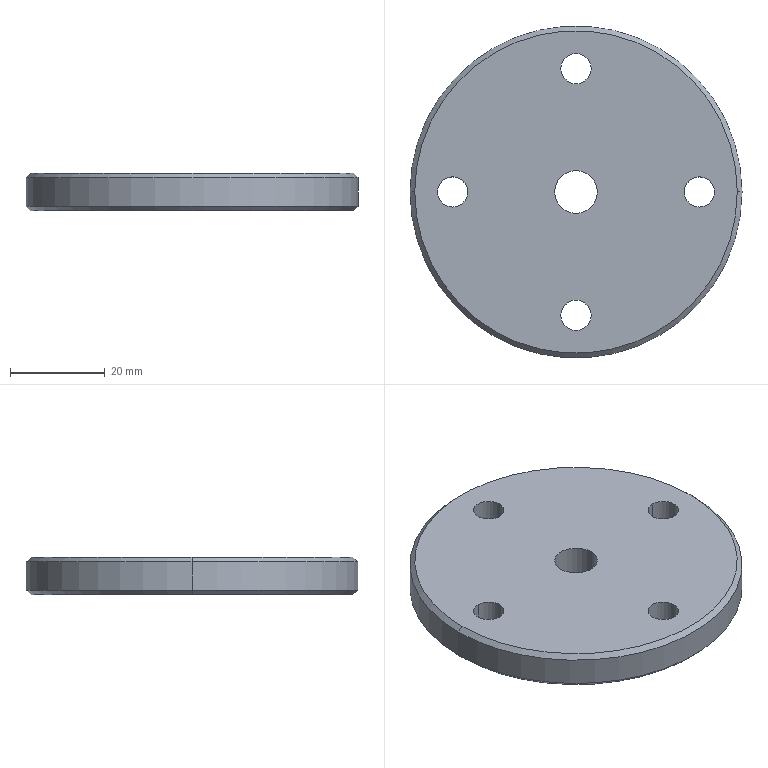Part | NX | features BREP 1 | 1 solid | 18 faces | box 70 x 70 x 8 mm | volume 29031 mm3 | cylinder 12 | cone 4 | plane 2 | commonest cylinder face diameters 6.4 x8 9 x2 70 x2
STEP:
#1=CARTESIAN_POINT('',(3.2,-26.,8.));
#2=VERTEX_POINT('',#1);
#3=CARTESIAN_POINT('',(-3.2,-26.,8.));
#4=VERTEX_POINT('',#3);
#5=CARTESIAN_POINT('',(0.,-26.,8.));
#6=DIRECTION('',(0.,0.,-1.));
#7=DIRECTION('',(1.,0.,0.));
#8=AXIS2_PLACEMENT_3D('',#5,#6,#7);
#9=CIRCLE('',#8,3.2);
#10=EDGE_CURVE('',#2,#4,#9,.T.);
#11=ORIENTED_EDGE('',*,*,#10,.F.);
#12=CARTESIAN_POINT('',(3.2,-26.,0.));
#13=VERTEX_POINT('',#12);
#14=CARTESIAN_POINT('',(3.2,-26.,0.));
#15=DIRECTION('',(0.,0.,1.));
#16=VECTOR('',#15,1000.);
#17=LINE('',#14,#16);
#18=EDGE_CURVE('',#2,#13,#17,.F.);
#19=ORIENTED_EDGE('',*,*,#18,.T.);
#20=CARTESIAN_POINT('',(-3.2,-26.,0.));
#21=VERTEX_POINT('',#20);
#22=CARTESIAN_POINT('',(0.,-26.,0.));
#23=DIRECTION('',(0.,0.,1.));
#24=DIRECTION('',(-1.,0.,0.));
#25=AXIS2_PLACEMENT_3D('',#22,#23,#24);
#26=CIRCLE('',#25,3.2);
#27=EDGE_CURVE('',#21,#13,#26,.T.);
#28=ORIENTED_EDGE('',*,*,#27,.F.);
#29=CARTESIAN_POINT('',(-3.2,-26.,0.));
#30=DIRECTION('',(0.,0.,1.));
#31=VECTOR('',#30,1000.);
#32=LINE('',#29,#31);
#33=EDGE_CURVE('',#4,#21,#32,.F.);
#34=ORIENTED_EDGE('',*,*,#33,.F.);
#35=EDGE_LOOP('',(#11,#19,#28,#34));
#36=FACE_BOUND('',#35,.T.);
#37=CARTESIAN_POINT('',(0.,-26.,0.));
#38=DIRECTION('',(0.,0.,1.));
#39=DIRECTION('',(1.,0.,0.));
#40=AXIS2_PLACEMENT_3D('',#37,#38,#39);
#41=CYLINDRICAL_SURFACE('',#40,3.2);
#42=ADVANCED_FACE('',(#36),#41,.F.);
#43=CARTESIAN_POINT('',(0.,-26.,8.));
#44=DIRECTION('',(0.,0.,-1.));
#45=DIRECTION('',(-1.,0.,0.));
#46=AXIS2_PLACEMENT_3D('',#43,#44,#45);
#47=CIRCLE('',#46,3.2);
#48=EDGE_CURVE('',#4,#2,#47,.T.);
#49=ORIENTED_EDGE('',*,*,#48,.F.);
#50=ORIENTED_EDGE('',*,*,#33,.T.);
#51=CARTESIAN_POINT('',(0.,-26.,0.));
#52=DIRECTION('',(0.,0.,1.));
#53=DIRECTION('',(1.,0.,0.));
#54=AXIS2_PLACEMENT_3D('',#51,#52,#53);
#55=CIRCLE('',#54,3.2);
#56=EDGE_CURVE('',#13,#21,#55,.T.);
#57=ORIENTED_EDGE('',*,*,#56,.F.);
#58=ORIENTED_EDGE('',*,*,#18,.F.);
#59=EDGE_LOOP('',(#49,#50,#57,#58));
#60=FACE_BOUND('',#59,.T.);
#61=CARTESIAN_POINT('',(0.,-26.,0.));
#62=DIRECTION('',(0.,0.,1.));
#63=DIRECTION('',(1.,0.,0.));
#64=AXIS2_PLACEMENT_3D('',#61,#62,#63);
#65=CYLINDRICAL_SURFACE('',#64,3.2);
#66=ADVANCED_FACE('',(#60),#65,.F.);
#67=CARTESIAN_POINT('',(34.,-0.000000001,0.));
#68=VERTEX_POINT('',#67);
#69=CARTESIAN_POINT('',(-34.,0.,0.));
#70=VERTEX_POINT('',#69);
#71=CARTESIAN_POINT('',(0.,0.,0.));
#72=DIRECTION('',(0.,0.,-1.));
#73=DIRECTION('',(0.5,-0.866,0.));
#74=AXIS2_PLACEMENT_3D('',#71,#72,#73);
#75=CIRCLE('',#74,34.);
#76=EDGE_CURVE('',#68,#70,#75,.T.);
#77=ORIENTED_EDGE('',*,*,#76,.T.);
#78=CARTESIAN_POINT('',(0.,0.,0.));
#79=DIRECTION('',(0.,0.,-1.));
#80=DIRECTION('',(-1.,0.,0.));
#81=AXIS2_PLACEMENT_3D('',#78,#79,#80);
#82=CIRCLE('',#81,34.);
#83=EDGE_CURVE('',#70,#68,#82,.T.);
#84=ORIENTED_EDGE('',*,*,#83,.T.);
#85=EDGE_LOOP('',(#77,#84));
#86=FACE_BOUND('',#85,.T.);
#87=ORIENTED_EDGE('',*,*,#56,.T.);
#88=ORIENTED_EDGE('',*,*,#27,.T.);
#89=EDGE_LOOP('',(#87,#88));
#90=FACE_BOUND('',#89,.T.);
#91=CARTESIAN_POINT('',(4.5,0.,0.));
#92=VERTEX_POINT('',#91);
#93=CARTESIAN_POINT('',(-4.5,0.,0.));
#94=VERTEX_POINT('',#93);
#95=CARTESIAN_POINT('',(0.,0.,0.));
#96=DIRECTION('',(0.,0.,1.));
#97=DIRECTION('',(1.,0.,0.));
#98=AXIS2_PLACEMENT_3D('',#95,#96,#97);
#99=CIRCLE('',#98,4.5);
#100=EDGE_CURVE('',#92,#94,#99,.T.);
#101=ORIENTED_EDGE('',*,*,#100,.T.);
#102=CARTESIAN_POINT('',(0.,0.,0.));
#103=DIRECTION('',(0.,0.,1.));
#104=DIRECTION('',(-1.,0.,0.));
#105=AXIS2_PLACEMENT_3D('',#102,#103,#104);
#106=CIRCLE('',#105,4.5);
#107=EDGE_CURVE('',#94,#92,#106,.T.);
#108=ORIENTED_EDGE('',*,*,#107,.T.);
#109=EDGE_LOOP('',(#101,#108));
#110=FACE_BOUND('',#109,.T.);
#111=CARTESIAN_POINT('',(26.,3.2,0.));
#112=VERTEX_POINT('',#111);
#113=CARTESIAN_POINT('',(26.,-3.2,0.));
#114=VERTEX_POINT('',#113);
#115=CARTESIAN_POINT('',(26.,0.,0.));
#116=DIRECTION('',(0.,0.,1.));
#117=DIRECTION('',(-1.,0.,0.));
#118=AXIS2_PLACEMENT_3D('',#115,#116,#117);
#119=CIRCLE('',#118,3.2);
#120=EDGE_CURVE('',#112,#114,#119,.T.);
#121=ORIENTED_EDGE('',*,*,#120,.T.);
#122=CARTESIAN_POINT('',(26.,0.,0.));
#123=DIRECTION('',(0.,0.,1.));
#124=DIRECTION('',(0.,-1.,0.));
#125=AXIS2_PLACEMENT_3D('',#122,#123,#124);
#126=CIRCLE('',#125,3.2);
#127=EDGE_CURVE('',#114,#112,#126,.T.);
#128=ORIENTED_EDGE('',*,*,#127,.T.);
#129=EDGE_LOOP('',(#121,#128));
#130=FACE_BOUND('',#129,.T.);
#131=CARTESIAN_POINT('',(3.2,26.,0.));
#132=VERTEX_POINT('',#131);
#133=CARTESIAN_POINT('',(-3.2,26.,0.));
#134=VERTEX_POINT('',#133);
#135=CARTESIAN_POINT('',(0.,26.,0.));
#136=DIRECTION('',(0.,0.,1.));
#137=DIRECTION('',(1.,0.,0.));
#138=AXIS2_PLACEMENT_3D('',#135,#136,#137);
#139=CIRCLE('',#138,3.2);
#140=EDGE_CURVE('',#132,#134,#139,.T.);
#141=ORIENTED_EDGE('',*,*,#140,.T.);
#142=CARTESIAN_POINT('',(0.,26.,0.));
#143=DIRECTION('',(0.,0.,1.));
#144=DIRECTION('',(-1.,0.,0.));
#145=AXIS2_PLACEMENT_3D('',#142,#143,#144);
#146=CIRCLE('',#145,3.2);
#147=EDGE_CURVE('',#134,#132,#146,.T.);
#148=ORIENTED_EDGE('',*,*,#147,.T.);
#149=EDGE_LOOP('',(#141,#148));
#150=FACE_BOUND('',#149,.T.);
#151=CARTESIAN_POINT('',(-26.,3.2,0.));
#152=VERTEX_POINT('',#151);
#153=CARTESIAN_POINT('',(-26.,-3.2,0.));
#154=VERTEX_POINT('',#153);
#155=CARTESIAN_POINT('',(-26.,0.,0.));
#156=DIRECTION('',(0.,0.,1.));
#157=DIRECTION('',(0.,1.,0.));
#158=AXIS2_PLACEMENT_3D('',#155,#156,#157);
#159=CIRCLE('',#158,3.2);
#160=EDGE_CURVE('',#152,#154,#159,.T.);
#161=ORIENTED_EDGE('',*,*,#160,.T.);
#162=CARTESIAN_POINT('',(-26.,0.,0.));
#163=DIRECTION('',(0.,0.,1.));
#164=DIRECTION('',(0.,-1.,0.));
#165=AXIS2_PLACEMENT_3D('',#162,#163,#164);
#166=CIRCLE('',#165,3.2);
#167=EDGE_CURVE('',#154,#152,#166,.T.);
#168=ORIENTED_EDGE('',*,*,#167,.T.);
#169=EDGE_LOOP('',(#161,#168));
#170=FACE_BOUND('',#169,.T.);
#171=CARTESIAN_POINT('',(0.,0.,0.));
#172=DIRECTION('',(0.,0.,1.));
#173=DIRECTION('',(1.,0.,0.));
#174=AXIS2_PLACEMENT_3D('',#171,#172,#173);
#175=PLANE('',#174);
#176=ADVANCED_FACE('',(#86,#90,#110,#130,#150,#170),#175,.F.);
#177=CARTESIAN_POINT('',(35.,0.,1.));
#178=VERTEX_POINT('',#177);
#179=CARTESIAN_POINT('',(35.,0.,1.));
#180=DIRECTION('',(-0.7071,0.,-0.7071));
#181=VECTOR('',#180,1000.);
#182=LINE('',#179,#181);
#183=EDGE_CURVE('',#68,#178,#182,.F.);
#184=ORIENTED_EDGE('',*,*,#183,.T.);
#185=CARTESIAN_POINT('',(-35.,0.,1.));
#186=VERTEX_POINT('',#185);
#187=CARTESIAN_POINT('',(0.,0.,1.));
#188=DIRECTION('',(0.,0.,-1.));
#189=DIRECTION('',(1.,0.,0.));
#190=AXIS2_PLACEMENT_3D('',#187,#188,#189);
#191=CIRCLE('',#190,35.);
#192=EDGE_CURVE('',#178,#186,#191,.T.);
#193=ORIENTED_EDGE('',*,*,#192,.T.);
#194=CARTESIAN_POINT('',(-35.,0.,1.));
#195=DIRECTION('',(0.7071,0.,-0.7071));
#196=VECTOR('',#195,1000.);
#197=LINE('',#194,#196);
#198=EDGE_CURVE('',#70,#186,#197,.F.);
#199=ORIENTED_EDGE('',*,*,#198,.F.);
#200=ORIENTED_EDGE('',*,*,#76,.F.);
#201=EDGE_LOOP('',(#184,#193,#199,#200));
#202=FACE_BOUND('',#201,.T.);
#203=CARTESIAN_POINT('',(0.,0.,0.5));
#204=DIRECTION('',(0.,0.,1.));
#205=DIRECTION('',(1.,0.,0.));
#206=AXIS2_PLACEMENT_3D('',#203,#204,#205);
#207=CONICAL_SURFACE('',#206,34.5,0.7854);
#208=ADVANCED_FACE('',(#202),#207,.T.);
#209=ORIENTED_EDGE('',*,*,#83,.F.);
#210=ORIENTED_EDGE('',*,*,#198,.T.);
#211=CARTESIAN_POINT('',(0.,0.,1.));
#212=DIRECTION('',(0.,0.,-1.));
#213=DIRECTION('',(-1.,0.,0.));
#214=AXIS2_PLACEMENT_3D('',#211,#212,#213);
#215=CIRCLE('',#214,35.);
#216=EDGE_CURVE('',#186,#178,#215,.T.);
#217=ORIENTED_EDGE('',*,*,#216,.T.);
#218=ORIENTED_EDGE('',*,*,#183,.F.);
#219=EDGE_LOOP('',(#209,#210,#217,#218));
#220=FACE_BOUND('',#219,.T.);
#221=CARTESIAN_POINT('',(0.,0.,0.5));
#222=DIRECTION('',(0.,0.,1.));
#223=DIRECTION('',(1.,0.,0.));
#224=AXIS2_PLACEMENT_3D('',#221,#222,#223);
#225=CONICAL_SURFACE('',#224,34.5,0.7854);
#226=ADVANCED_FACE('',(#220),#225,.T.);
#227=ORIENTED_EDGE('',*,*,#216,.F.);
#228=CARTESIAN_POINT('',(-35.,0.,7.));
#229=VERTEX_POINT('',#228);
#230=CARTESIAN_POINT('',(-35.,0.,7.));
#231=DIRECTION('',(0.,0.,-1.));
#232=VECTOR('',#231,1000.);
#233=LINE('',#230,#232);
#234=EDGE_CURVE('',#186,#229,#233,.F.);
#235=ORIENTED_EDGE('',*,*,#234,.T.);
#236=CARTESIAN_POINT('',(35.,0.,7.));
#237=VERTEX_POINT('',#236);
#238=CARTESIAN_POINT('',(0.,0.,7.));
#239=DIRECTION('',(0.,0.,1.));
#240=DIRECTION('',(1.,0.,0.));
#241=AXIS2_PLACEMENT_3D('',#238,#239,#240);
#242=CIRCLE('',#241,35.);
#243=EDGE_CURVE('',#237,#229,#242,.T.);
#244=ORIENTED_EDGE('',*,*,#243,.F.);
#245=CARTESIAN_POINT('',(35.,0.,7.));
#246=DIRECTION('',(0.,0.,-1.));
#247=VECTOR('',#246,1000.);
#248=LINE('',#245,#247);
#249=EDGE_CURVE('',#178,#237,#248,.F.);
#250=ORIENTED_EDGE('',*,*,#249,.F.);
#251=EDGE_LOOP('',(#227,#235,#244,#250));
#252=FACE_BOUND('',#251,.T.);
#253=CARTESIAN_POINT('',(0.,0.,4.));
#254=DIRECTION('',(0.,0.,1.));
#255=DIRECTION('',(1.,0.,0.));
#256=AXIS2_PLACEMENT_3D('',#253,#254,#255);
#257=CYLINDRICAL_SURFACE('',#256,35.);
#258=ADVANCED_FACE('',(#252),#257,.T.);
#259=ORIENTED_EDGE('',*,*,#234,.F.);
#260=ORIENTED_EDGE('',*,*,#192,.F.);
#261=ORIENTED_EDGE('',*,*,#249,.T.);
#262=CARTESIAN_POINT('',(0.,0.,7.));
#263=DIRECTION('',(0.,0.,1.));
#264=DIRECTION('',(0.5,-0.866,0.));
#265=AXIS2_PLACEMENT_3D('',#262,#263,#264);
#266=CIRCLE('',#265,35.);
#267=EDGE_CURVE('',#229,#237,#266,.T.);
#268=ORIENTED_EDGE('',*,*,#267,.F.);
#269=EDGE_LOOP('',(#259,#260,#261,#268));
#270=FACE_BOUND('',#269,.T.);
#271=CARTESIAN_POINT('',(0.,0.,4.));
#272=DIRECTION('',(0.,0.,1.));
#273=DIRECTION('',(1.,0.,0.));
#274=AXIS2_PLACEMENT_3D('',#271,#272,#273);
#275=CYLINDRICAL_SURFACE('',#274,35.);
#276=ADVANCED_FACE('',(#270),#275,.T.);
#277=CARTESIAN_POINT('',(-34.,0.,8.));
#278=VERTEX_POINT('',#277);
#279=CARTESIAN_POINT('',(-34.,0.,8.));
#280=DIRECTION('',(-0.7071,0.,-0.7071));
#281=VECTOR('',#280,1000.);
#282=LINE('',#279,#281);
#283=EDGE_CURVE('',#278,#229,#282,.T.);
#284=ORIENTED_EDGE('',*,*,#283,.T.);
#285=ORIENTED_EDGE('',*,*,#267,.T.);
#286=CARTESIAN_POINT('',(34.,0.,8.));
#287=VERTEX_POINT('',#286);
#288=CARTESIAN_POINT('',(35.,0.,7.));
#289=DIRECTION('',(-0.7071,0.,0.7071));
#290=VECTOR('',#289,1000.);
#291=LINE('',#288,#290);
#292=EDGE_CURVE('',#237,#287,#291,.T.);
#293=ORIENTED_EDGE('',*,*,#292,.T.);
#294=CARTESIAN_POINT('',(0.,0.,8.));
#295=DIRECTION('',(0.,0.,1.));
#296=DIRECTION('',(0.5,-0.866,0.));
#297=AXIS2_PLACEMENT_3D('',#294,#295,#296);
#298=CIRCLE('',#297,34.);
#299=EDGE_CURVE('',#278,#287,#298,.T.);
#300=ORIENTED_EDGE('',*,*,#299,.F.);
#301=EDGE_LOOP('',(#284,#285,#293,#300));
#302=FACE_BOUND('',#301,.T.);
#303=CARTESIAN_POINT('',(0.,0.,7.5));
#304=DIRECTION('',(0.,0.,-1.));
#305=DIRECTION('',(1.,0.,0.));
#306=AXIS2_PLACEMENT_3D('',#303,#304,#305);
#307=CONICAL_SURFACE('',#306,34.5,0.7854);
#308=ADVANCED_FACE('',(#302),#307,.T.);
#309=CARTESIAN_POINT('',(0.,0.,8.));
#310=DIRECTION('',(0.,0.,1.));
#311=DIRECTION('',(1.,0.,0.));
#312=AXIS2_PLACEMENT_3D('',#309,#310,#311);
#313=CIRCLE('',#312,34.);
#314=EDGE_CURVE('',#287,#278,#313,.T.);
#315=ORIENTED_EDGE('',*,*,#314,.T.);
#316=ORIENTED_EDGE('',*,*,#299,.T.);
#317=EDGE_LOOP('',(#315,#316));
#318=FACE_BOUND('',#317,.T.);
#319=ORIENTED_EDGE('',*,*,#10,.T.);
#320=ORIENTED_EDGE('',*,*,#48,.T.);
#321=EDGE_LOOP('',(#319,#320));
#322=FACE_BOUND('',#321,.T.);
#323=CARTESIAN_POINT('',(4.5,0.,8.));
#324=VERTEX_POINT('',#323);
#325=CARTESIAN_POINT('',(-4.5,0.,8.));
#326=VERTEX_POINT('',#325);
#327=CARTESIAN_POINT('',(0.,0.,8.));
#328=DIRECTION('',(0.,0.,-1.));
#329=DIRECTION('',(1.,0.,0.));
#330=AXIS2_PLACEMENT_3D('',#327,#328,#329);
#331=CIRCLE('',#330,4.5);
#332=EDGE_CURVE('',#324,#326,#331,.T.);
#333=ORIENTED_EDGE('',*,*,#332,.T.);
#334=CARTESIAN_POINT('',(0.,0.,8.));
#335=DIRECTION('',(0.,0.,-1.));
#336=DIRECTION('',(-1.,0.,0.));
#337=AXIS2_PLACEMENT_3D('',#334,#335,#336);
#338=CIRCLE('',#337,4.5);
#339=EDGE_CURVE('',#326,#324,#338,.T.);
#340=ORIENTED_EDGE('',*,*,#339,.T.);
#341=EDGE_LOOP('',(#333,#340));
#342=FACE_BOUND('',#341,.T.);
#343=CARTESIAN_POINT('',(26.,-3.2,8.));
#344=VERTEX_POINT('',#343);
#345=CARTESIAN_POINT('',(26.,3.2,8.));
#346=VERTEX_POINT('',#345);
#347=CARTESIAN_POINT('',(26.,0.,8.));
#348=DIRECTION('',(0.,0.,-1.));
#349=DIRECTION('',(0.,-1.,0.));
#350=AXIS2_PLACEMENT_3D('',#347,#348,#349);
#351=CIRCLE('',#350,3.2);
#352=EDGE_CURVE('',#344,#346,#351,.T.);
#353=ORIENTED_EDGE('',*,*,#352,.T.);
#354=CARTESIAN_POINT('',(26.,0.,8.));
#355=DIRECTION('',(0.,0.,-1.));
#356=DIRECTION('',(0.,1.,0.));
#357=AXIS2_PLACEMENT_3D('',#354,#355,#356);
#358=CIRCLE('',#357,3.2);
#359=EDGE_CURVE('',#346,#344,#358,.T.);
#360=ORIENTED_EDGE('',*,*,#359,.T.);
#361=EDGE_LOOP('',(#353,#360));
#362=FACE_BOUND('',#361,.T.);
#363=CARTESIAN_POINT('',(3.2,26.,8.));
#364=VERTEX_POINT('',#363);
#365=CARTESIAN_POINT('',(-3.2,26.,8.));
#366=VERTEX_POINT('',#365);
#367=CARTESIAN_POINT('',(0.,26.,8.));
#368=DIRECTION('',(0.,0.,-1.));
#369=DIRECTION('',(1.,0.,0.));
#370=AXIS2_PLACEMENT_3D('',#367,#368,#369);
#371=CIRCLE('',#370,3.2);
#372=EDGE_CURVE('',#364,#366,#371,.T.);
#373=ORIENTED_EDGE('',*,*,#372,.T.);
#374=CARTESIAN_POINT('',(0.,26.,8.));
#375=DIRECTION('',(0.,0.,-1.));
#376=DIRECTION('',(-1.,0.,0.));
#377=AXIS2_PLACEMENT_3D('',#374,#375,#376);
#378=CIRCLE('',#377,3.2);
#379=EDGE_CURVE('',#366,#364,#378,.T.);
#380=ORIENTED_EDGE('',*,*,#379,.T.);
#381=EDGE_LOOP('',(#373,#380));
#382=FACE_BOUND('',#381,.T.);
#383=CARTESIAN_POINT('',(-26.,3.2,8.));
#384=VERTEX_POINT('',#383);
#385=CARTESIAN_POINT('',(-26.,-3.2,8.));
#386=VERTEX_POINT('',#385);
#387=CARTESIAN_POINT('',(-26.,0.,8.));
#388=DIRECTION('',(0.,0.,-1.));
#389=DIRECTION('',(0.,1.,0.));
#390=AXIS2_PLACEMENT_3D('',#387,#388,#389);
#391=CIRCLE('',#390,3.2);
#392=EDGE_CURVE('',#384,#386,#391,.T.);
#393=ORIENTED_EDGE('',*,*,#392,.T.);
#394=CARTESIAN_POINT('',(-26.,0.,8.));
#395=DIRECTION('',(0.,0.,-1.));
#396=DIRECTION('',(0.,-1.,0.));
#397=AXIS2_PLACEMENT_3D('',#394,#395,#396);
#398=CIRCLE('',#397,3.2);
#399=EDGE_CURVE('',#386,#384,#398,.T.);
#400=ORIENTED_EDGE('',*,*,#399,.T.);
#401=EDGE_LOOP('',(#393,#400));
#402=FACE_BOUND('',#401,.T.);
#403=CARTESIAN_POINT('',(0.,0.,8.));
#404=DIRECTION('',(0.,0.,1.));
#405=DIRECTION('',(1.,0.,0.));
#406=AXIS2_PLACEMENT_3D('',#403,#404,#405);
#407=PLANE('',#406);
#408=ADVANCED_FACE('',(#318,#322,#342,#362,#382,#402),#407,.T.);
#409=ORIENTED_EDGE('',*,*,#243,.T.);
#410=ORIENTED_EDGE('',*,*,#283,.F.);
#411=ORIENTED_EDGE('',*,*,#314,.F.);
#412=ORIENTED_EDGE('',*,*,#292,.F.);
#413=EDGE_LOOP('',(#409,#410,#411,#412));
#414=FACE_BOUND('',#413,.T.);
#415=CARTESIAN_POINT('',(0.,0.,7.5));
#416=DIRECTION('',(0.,0.,-1.));
#417=DIRECTION('',(1.,0.,0.));
#418=AXIS2_PLACEMENT_3D('',#415,#416,#417);
#419=CONICAL_SURFACE('',#418,34.5,0.7854);
#420=ADVANCED_FACE('',(#414),#419,.T.);
#421=ORIENTED_EDGE('',*,*,#339,.F.);
#422=CARTESIAN_POINT('',(-4.5,0.,0.));
#423=DIRECTION('',(0.,0.,1.));
#424=VECTOR('',#423,1000.);
#425=LINE('',#422,#424);
#426=EDGE_CURVE('',#94,#326,#425,.T.);
#427=ORIENTED_EDGE('',*,*,#426,.F.);
#428=ORIENTED_EDGE('',*,*,#100,.F.);
#429=CARTESIAN_POINT('',(4.5,0.,0.));
#430=DIRECTION('',(0.,0.,1.));
#431=VECTOR('',#430,1000.);
#432=LINE('',#429,#431);
#433=EDGE_CURVE('',#92,#324,#432,.T.);
#434=ORIENTED_EDGE('',*,*,#433,.T.);
#435=EDGE_LOOP('',(#421,#427,#428,#434));
#436=FACE_BOUND('',#435,.T.);
#437=CARTESIAN_POINT('',(0.,0.,0.));
#438=DIRECTION('',(0.,0.,1.));
#439=DIRECTION('',(1.,0.,0.));
#440=AXIS2_PLACEMENT_3D('',#437,#438,#439);
#441=CYLINDRICAL_SURFACE('',#440,4.5);
#442=ADVANCED_FACE('',(#436),#441,.F.);
#443=ORIENTED_EDGE('',*,*,#332,.F.);
#444=ORIENTED_EDGE('',*,*,#433,.F.);
#445=ORIENTED_EDGE('',*,*,#107,.F.);
#446=ORIENTED_EDGE('',*,*,#426,.T.);
#447=EDGE_LOOP('',(#443,#444,#445,#446));
#448=FACE_BOUND('',#447,.T.);
#449=CARTESIAN_POINT('',(0.,0.,0.));
#450=DIRECTION('',(0.,0.,1.));
#451=DIRECTION('',(1.,0.,0.));
#452=AXIS2_PLACEMENT_3D('',#449,#450,#451);
#453=CYLINDRICAL_SURFACE('',#452,4.5);
#454=ADVANCED_FACE('',(#448),#453,.F.);
#455=ORIENTED_EDGE('',*,*,#359,.F.);
#456=CARTESIAN_POINT('',(26.,3.2,0.));
#457=DIRECTION('',(0.,0.,1.));
#458=VECTOR('',#457,1000.);
#459=LINE('',#456,#458);
#460=EDGE_CURVE('',#346,#112,#459,.F.);
#461=ORIENTED_EDGE('',*,*,#460,.T.);
#462=ORIENTED_EDGE('',*,*,#127,.F.);
#463=CARTESIAN_POINT('',(26.,-3.2,0.));
#464=DIRECTION('',(0.,0.,1.));
#465=VECTOR('',#464,1000.);
#466=LINE('',#463,#465);
#467=EDGE_CURVE('',#344,#114,#466,.F.);
#468=ORIENTED_EDGE('',*,*,#467,.F.);
#469=EDGE_LOOP('',(#455,#461,#462,#468));
#470=FACE_BOUND('',#469,.T.);
#471=CARTESIAN_POINT('',(26.,0.,0.));
#472=DIRECTION('',(0.,0.,1.));
#473=DIRECTION('',(0.,1.,0.));
#474=AXIS2_PLACEMENT_3D('',#471,#472,#473);
#475=CYLINDRICAL_SURFACE('',#474,3.2);
#476=ADVANCED_FACE('',(#470),#475,.F.);
#477=ORIENTED_EDGE('',*,*,#352,.F.);
#478=ORIENTED_EDGE('',*,*,#467,.T.);
#479=ORIENTED_EDGE('',*,*,#120,.F.);
#480=ORIENTED_EDGE('',*,*,#460,.F.);
#481=EDGE_LOOP('',(#477,#478,#479,#480));
#482=FACE_BOUND('',#481,.T.);
#483=CARTESIAN_POINT('',(26.,0.,0.));
#484=DIRECTION('',(0.,0.,1.));
#485=DIRECTION('',(0.,1.,0.));
#486=AXIS2_PLACEMENT_3D('',#483,#484,#485);
#487=CYLINDRICAL_SURFACE('',#486,3.2);
#488=ADVANCED_FACE('',(#482),#487,.F.);
#489=ORIENTED_EDGE('',*,*,#379,.F.);
#490=CARTESIAN_POINT('',(-3.2,26.,0.));
#491=DIRECTION('',(0.,0.,1.));
#492=VECTOR('',#491,1000.);
#493=LINE('',#490,#492);
#494=EDGE_CURVE('',#134,#366,#493,.T.);
#495=ORIENTED_EDGE('',*,*,#494,.F.);
#496=ORIENTED_EDGE('',*,*,#140,.F.);
#497=CARTESIAN_POINT('',(3.2,26.,0.));
#498=DIRECTION('',(0.,0.,1.));
#499=VECTOR('',#498,1000.);
#500=LINE('',#497,#499);
#501=EDGE_CURVE('',#132,#364,#500,.T.);
#502=ORIENTED_EDGE('',*,*,#501,.T.);
#503=EDGE_LOOP('',(#489,#495,#496,#502));
#504=FACE_BOUND('',#503,.T.);
#505=CARTESIAN_POINT('',(0.,26.,0.));
#506=DIRECTION('',(0.,0.,1.));
#507=DIRECTION('',(-1.,0.,0.));
#508=AXIS2_PLACEMENT_3D('',#505,#506,#507);
#509=CYLINDRICAL_SURFACE('',#508,3.2);
#510=ADVANCED_FACE('',(#504),#509,.F.);
#511=ORIENTED_EDGE('',*,*,#372,.F.);
#512=ORIENTED_EDGE('',*,*,#501,.F.);
#513=ORIENTED_EDGE('',*,*,#147,.F.);
#514=ORIENTED_EDGE('',*,*,#494,.T.);
#515=EDGE_LOOP('',(#511,#512,#513,#514));
#516=FACE_BOUND('',#515,.T.);
#517=CARTESIAN_POINT('',(0.,26.,0.));
#518=DIRECTION('',(0.,0.,1.));
#519=DIRECTION('',(-1.,0.,0.));
#520=AXIS2_PLACEMENT_3D('',#517,#518,#519);
#521=CYLINDRICAL_SURFACE('',#520,3.2);
#522=ADVANCED_FACE('',(#516),#521,.F.);
#523=ORIENTED_EDGE('',*,*,#399,.F.);
#524=CARTESIAN_POINT('',(-26.,-3.2,0.));
#525=DIRECTION('',(0.,0.,1.));
#526=VECTOR('',#525,1000.);
#527=LINE('',#524,#526);
#528=EDGE_CURVE('',#154,#386,#527,.T.);
#529=ORIENTED_EDGE('',*,*,#528,.F.);
#530=ORIENTED_EDGE('',*,*,#160,.F.);
#531=CARTESIAN_POINT('',(-26.,3.2,0.));
#532=DIRECTION('',(0.,0.,1.));
#533=VECTOR('',#532,1000.);
#534=LINE('',#531,#533);
#535=EDGE_CURVE('',#152,#384,#534,.T.);
#536=ORIENTED_EDGE('',*,*,#535,.T.);
#537=EDGE_LOOP('',(#523,#529,#530,#536));
#538=FACE_BOUND('',#537,.T.);
#539=CARTESIAN_POINT('',(-26.,0.,0.));
#540=DIRECTION('',(0.,0.,1.));
#541=DIRECTION('',(0.,-1.,0.));
#542=AXIS2_PLACEMENT_3D('',#539,#540,#541);
#543=CYLINDRICAL_SURFACE('',#542,3.2);
#544=ADVANCED_FACE('',(#538),#543,.F.);
#545=ORIENTED_EDGE('',*,*,#392,.F.);
#546=ORIENTED_EDGE('',*,*,#535,.F.);
#547=ORIENTED_EDGE('',*,*,#167,.F.);
#548=ORIENTED_EDGE('',*,*,#528,.T.);
#549=EDGE_LOOP('',(#545,#546,#547,#548));
#550=FACE_BOUND('',#549,.T.);
#551=CARTESIAN_POINT('',(-26.,0.,0.));
#552=DIRECTION('',(0.,0.,1.));
#553=DIRECTION('',(0.,-1.,0.));
#554=AXIS2_PLACEMENT_3D('',#551,#552,#553);
#555=CYLINDRICAL_SURFACE('',#554,3.2);
#556=ADVANCED_FACE('',(#550),#555,.F.);
#557=CLOSED_SHELL('',(#42,#66,#176,#208,#226,#258,#276,#308,#408,#420,#442,#454,#476,#488,#510,#522,#544,#556));
#558=MANIFOLD_SOLID_BREP('',#557);
#559=(LENGTH_UNIT()NAMED_UNIT(*)SI_UNIT(.MILLI.,.METRE.));
#560=UNCERTAINTY_MEASURE_WITH_UNIT(LENGTH_MEASURE(0.00001),#559,'','');
#561=(NAMED_UNIT(*)PLANE_ANGLE_UNIT()SI_UNIT($,.RADIAN.));
#562=(NAMED_UNIT(*)SI_UNIT($,.STERADIAN.)SOLID_ANGLE_UNIT());
#563=(GEOMETRIC_REPRESENTATION_CONTEXT(3)GLOBAL_UNCERTAINTY_ASSIGNED_CONTEXT((#560))GLOBAL_UNIT_ASSIGNED_CONTEXT((#559,#561,#562))REPRESENTATION_CONTEXT('',''));
#564=ADVANCED_BREP_SHAPE_REPRESENTATION('',(#558),#563);